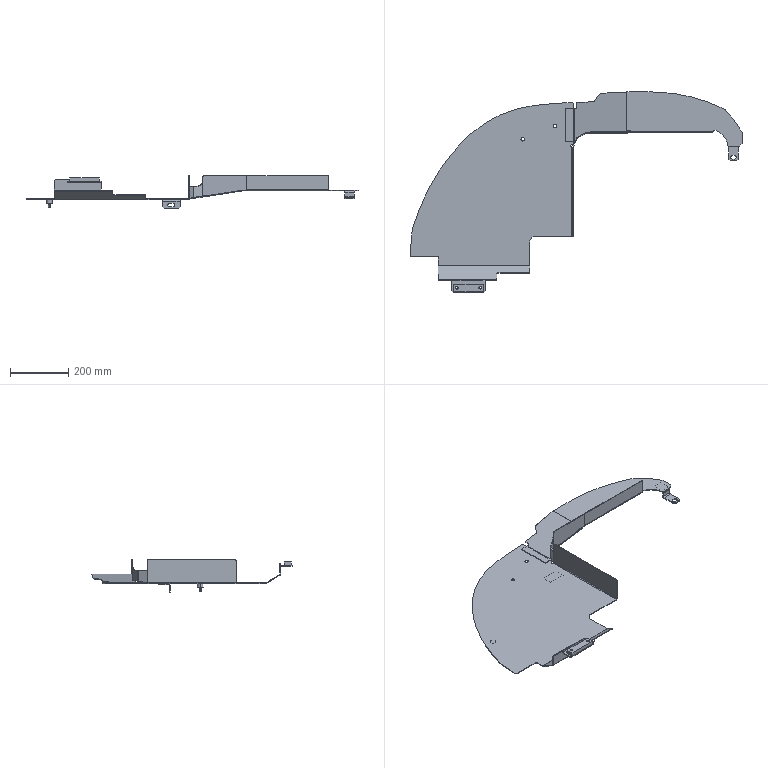Part | SolidWorks | features MBimport 1 | 8 solids | 208 faces | box 1139 x 687.3 x 112.3 mm | volume 932839 mm3 | plane 110 | cylinder 80 | spline 14 | torus 2 | cone 2 | commonest cylinder face diameters 10 x14 12.5 x9 4.6 x5 6 x5 9.2 x5 8 x4